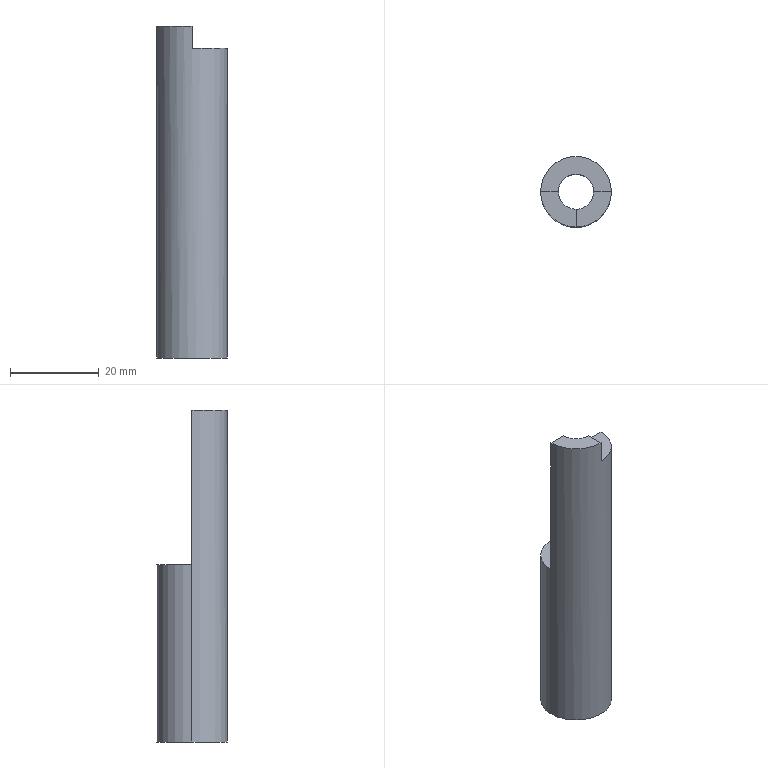Part | CATIA | 1 solid | 11 faces | box 16 x 16 x 75 mm | volume 8482 mm3 | plane 7 | cylinder 4 | commonest cylinder face diameters 8 x2 16 x2
STEP:
#1=CARTESIAN_POINT('',(-8.,0.,13.));
#2=VERTEX_POINT('',#1);
#3=CARTESIAN_POINT('',(8.,0.,13.));
#4=VERTEX_POINT('',#3);
#5=CARTESIAN_POINT('',(0.,0.,13.));
#6=DIRECTION('',(0.,0.,1.));
#7=AXIS2_PLACEMENT_3D('',#5,#6,$);
#8=CIRCLE('',#7,8.);
#9=EDGE_CURVE('',#2,#4,#8,.T.);
#10=ORIENTED_EDGE('',*,*,#9,.F.);
#11=CARTESIAN_POINT('',(0.,0.,13.));
#12=DIRECTION('',(0.,0.,1.));
#13=AXIS2_PLACEMENT_3D('',#11,#12,$);
#14=CIRCLE('',#13,8.);
#15=EDGE_CURVE('',#4,#2,#14,.T.);
#16=ORIENTED_EDGE('',*,*,#15,.F.);
#17=EDGE_LOOP('',(#10,#16));
#18=FACE_OUTER_BOUND('',#17,.T.);
#19=CARTESIAN_POINT('',(4.,0.,13.));
#20=VERTEX_POINT('',#19);
#21=CARTESIAN_POINT('',(-4.,0.,13.));
#22=VERTEX_POINT('',#21);
#23=CARTESIAN_POINT('',(0.,0.,13.));
#24=DIRECTION('',(0.,0.,1.));
#25=AXIS2_PLACEMENT_3D('',#23,#24,$);
#26=CIRCLE('',#25,4.);
#27=EDGE_CURVE('',#20,#22,#26,.T.);
#28=ORIENTED_EDGE('',*,*,#27,.T.);
#29=CARTESIAN_POINT('',(0.,0.,13.));
#30=DIRECTION('',(0.,0.,1.));
#31=AXIS2_PLACEMENT_3D('',#29,#30,$);
#32=CIRCLE('',#31,4.);
#33=EDGE_CURVE('',#22,#20,#32,.T.);
#34=ORIENTED_EDGE('',*,*,#33,.T.);
#35=EDGE_LOOP('',(#28,#34));
#36=FACE_BOUND('',#35,.T.);
#37=CARTESIAN_POINT('',(0.,0.,13.));
#38=DIRECTION('',(0.,0.,1.));
#39=DIRECTION('',(1.,0.,0.));
#40=AXIS2_PLACEMENT_3D('',#37,#38,#39);
#41=PLANE('',#40);
#42=ADVANCED_FACE('',(#18,#36),#41,.F.);
#43=CARTESIAN_POINT('',(4.,0.,53.));
#44=VERTEX_POINT('',#43);
#45=CARTESIAN_POINT('',(-4.,0.,53.));
#46=VERTEX_POINT('',#45);
#47=CARTESIAN_POINT('',(0.,0.,53.));
#48=DIRECTION('',(0.,0.,1.));
#49=AXIS2_PLACEMENT_3D('',#47,#48,$);
#50=CIRCLE('',#49,4.);
#51=EDGE_CURVE('',#44,#46,#50,.T.);
#52=ORIENTED_EDGE('',*,*,#51,.T.);
#53=CARTESIAN_POINT('',(-4.,0.,50.5));
#54=DIRECTION('',(0.,0.,1.));
#55=VECTOR('',#54,1.);
#56=LINE('',#53,#55);
#57=EDGE_CURVE('',#46,#22,#56,.F.);
#58=ORIENTED_EDGE('',*,*,#57,.T.);
#59=ORIENTED_EDGE('',*,*,#27,.F.);
#60=CARTESIAN_POINT('',(4.,0.,50.5));
#61=DIRECTION('',(0.,0.,1.));
#62=VECTOR('',#61,1.);
#63=LINE('',#60,#62);
#64=EDGE_CURVE('',#44,#20,#63,.F.);
#65=ORIENTED_EDGE('',*,*,#64,.F.);
#66=EDGE_LOOP('',(#52,#58,#59,#65));
#67=FACE_OUTER_BOUND('',#66,.T.);
#68=CARTESIAN_POINT('',(0.,0.,50.5));
#69=DIRECTION('',(0.,0.,1.));
#70=DIRECTION('',(1.,0.,0.));
#71=AXIS2_PLACEMENT_3D('',#68,#69,#70);
#72=CYLINDRICAL_SURFACE('',#71,4.);
#73=ADVANCED_FACE('',(#67),#72,.F.);
#74=CARTESIAN_POINT('',(8.,0.,53.));
#75=VERTEX_POINT('',#74);
#76=CARTESIAN_POINT('',(8.,0.,50.5));
#77=DIRECTION('',(0.,0.,1.));
#78=VECTOR('',#77,1.);
#79=LINE('',#76,#78);
#80=EDGE_CURVE('',#75,#4,#79,.F.);
#81=ORIENTED_EDGE('',*,*,#80,.T.);
#82=ORIENTED_EDGE('',*,*,#15,.T.);
#83=CARTESIAN_POINT('',(-8.,0.,53.));
#84=VERTEX_POINT('',#83);
#85=CARTESIAN_POINT('',(-8.,0.,50.5));
#86=DIRECTION('',(0.,0.,1.));
#87=VECTOR('',#86,1.);
#88=LINE('',#85,#87);
#89=EDGE_CURVE('',#84,#2,#88,.F.);
#90=ORIENTED_EDGE('',*,*,#89,.F.);
#91=CARTESIAN_POINT('',(0.,0.,53.));
#92=DIRECTION('',(0.,0.,1.));
#93=AXIS2_PLACEMENT_3D('',#91,#92,$);
#94=CIRCLE('',#93,8.);
#95=EDGE_CURVE('',#75,#84,#94,.T.);
#96=ORIENTED_EDGE('',*,*,#95,.F.);
#97=EDGE_LOOP('',(#81,#82,#90,#96));
#98=FACE_OUTER_BOUND('',#97,.T.);
#99=CARTESIAN_POINT('',(0.,0.,50.5));
#100=DIRECTION('',(0.,0.,1.));
#101=DIRECTION('',(1.,0.,0.));
#102=AXIS2_PLACEMENT_3D('',#99,#100,#101);
#103=CYLINDRICAL_SURFACE('',#102,8.);
#104=ADVANCED_FACE('',(#98),#103,.T.);
#105=ORIENTED_EDGE('',*,*,#51,.F.);
#106=CARTESIAN_POINT('',(6.,0.,53.));
#107=DIRECTION('',(1.,0.,0.));
#108=VECTOR('',#107,1.);
#109=LINE('',#106,#108);
#110=EDGE_CURVE('',#44,#75,#109,.T.);
#111=ORIENTED_EDGE('',*,*,#110,.T.);
#112=ORIENTED_EDGE('',*,*,#95,.T.);
#113=CARTESIAN_POINT('',(-6.,0.,53.));
#114=DIRECTION('',(1.,0.,0.));
#115=VECTOR('',#114,1.);
#116=LINE('',#113,#115);
#117=EDGE_CURVE('',#84,#46,#116,.T.);
#118=ORIENTED_EDGE('',*,*,#117,.T.);
#119=EDGE_LOOP('',(#105,#111,#112,#118));
#120=FACE_OUTER_BOUND('',#119,.T.);
#121=CARTESIAN_POINT('',(0.,0.,53.));
#122=DIRECTION('',(0.,0.,1.));
#123=DIRECTION('',(1.,0.,0.));
#124=AXIS2_PLACEMENT_3D('',#121,#122,#123);
#125=PLANE('',#124);
#126=ADVANCED_FACE('',(#120),#125,.T.);
#127=CARTESIAN_POINT('',(-4.,0.,88.));
#128=VERTEX_POINT('',#127);
#129=CARTESIAN_POINT('',(-4.,0.,70.5));
#130=DIRECTION('',(0.,0.,1.));
#131=VECTOR('',#130,1.);
#132=LINE('',#129,#131);
#133=EDGE_CURVE('',#128,#46,#132,.F.);
#134=ORIENTED_EDGE('',*,*,#133,.T.);
#135=ORIENTED_EDGE('',*,*,#117,.F.);
#136=CARTESIAN_POINT('',(-8.,0.,88.));
#137=VERTEX_POINT('',#136);
#138=CARTESIAN_POINT('',(-8.,0.,70.5));
#139=DIRECTION('',(0.,0.,1.));
#140=VECTOR('',#139,1.);
#141=LINE('',#138,#140);
#142=EDGE_CURVE('',#137,#84,#141,.F.);
#143=ORIENTED_EDGE('',*,*,#142,.F.);
#144=CARTESIAN_POINT('',(-6.,0.,88.));
#145=DIRECTION('',(1.,0.,0.));
#146=VECTOR('',#145,1.);
#147=LINE('',#144,#146);
#148=EDGE_CURVE('',#137,#128,#147,.T.);
#149=ORIENTED_EDGE('',*,*,#148,.T.);
#150=EDGE_LOOP('',(#134,#135,#143,#149));
#151=FACE_OUTER_BOUND('',#150,.T.);
#152=CARTESIAN_POINT('',(-12.734,0.,88.));
#153=DIRECTION('',(0.,1.,0.));
#154=DIRECTION('',(1.,0.,0.));
#155=AXIS2_PLACEMENT_3D('',#152,#153,#154);
#156=PLANE('',#155);
#157=ADVANCED_FACE('',(#151),#156,.T.);
#158=CARTESIAN_POINT('',(8.,0.,83.));
#159=VERTEX_POINT('',#158);
#160=CARTESIAN_POINT('',(8.,0.,68.));
#161=DIRECTION('',(0.,0.,1.));
#162=VECTOR('',#161,1.);
#163=LINE('',#160,#162);
#164=EDGE_CURVE('',#159,#75,#163,.F.);
#165=ORIENTED_EDGE('',*,*,#164,.T.);
#166=ORIENTED_EDGE('',*,*,#110,.F.);
#167=CARTESIAN_POINT('',(4.,0.,83.));
#168=VERTEX_POINT('',#167);
#169=CARTESIAN_POINT('',(4.,0.,68.));
#170=DIRECTION('',(0.,0.,1.));
#171=VECTOR('',#170,1.);
#172=LINE('',#169,#171);
#173=EDGE_CURVE('',#168,#44,#172,.F.);
#174=ORIENTED_EDGE('',*,*,#173,.F.);
#175=CARTESIAN_POINT('',(6.,0.,83.));
#176=DIRECTION('',(1.,0.,0.));
#177=VECTOR('',#176,1.);
#178=LINE('',#175,#177);
#179=EDGE_CURVE('',#168,#159,#178,.T.);
#180=ORIENTED_EDGE('',*,*,#179,.T.);
#181=EDGE_LOOP('',(#165,#166,#174,#180));
#182=FACE_OUTER_BOUND('',#181,.T.);
#183=ADVANCED_FACE('',(#182),#156,.T.);
#184=CARTESIAN_POINT('',(0.,-4.,88.));
#185=VERTEX_POINT('',#184);
#186=CARTESIAN_POINT('',(0.,0.,88.));
#187=DIRECTION('',(0.,0.,1.));
#188=AXIS2_PLACEMENT_3D('',#186,#187,$);
#189=CIRCLE('',#188,4.);
#190=EDGE_CURVE('',#128,#185,#189,.T.);
#191=ORIENTED_EDGE('',*,*,#190,.F.);
#192=ORIENTED_EDGE('',*,*,#148,.F.);
#193=CARTESIAN_POINT('',(0.,-8.,88.));
#194=VERTEX_POINT('',#193);
#195=CARTESIAN_POINT('',(0.,0.,88.));
#196=DIRECTION('',(0.,0.,1.));
#197=AXIS2_PLACEMENT_3D('',#195,#196,$);
#198=CIRCLE('',#197,8.);
#199=EDGE_CURVE('',#137,#194,#198,.T.);
#200=ORIENTED_EDGE('',*,*,#199,.T.);
#201=CARTESIAN_POINT('',(0.,-6.,88.));
#202=DIRECTION('',(0.,-1.,0.));
#203=VECTOR('',#202,1.);
#204=LINE('',#201,#203);
#205=EDGE_CURVE('',#185,#194,#204,.T.);
#206=ORIENTED_EDGE('',*,*,#205,.F.);
#207=EDGE_LOOP('',(#191,#192,#200,#206));
#208=FACE_OUTER_BOUND('',#207,.T.);
#209=CARTESIAN_POINT('',(0.,0.,88.));
#210=DIRECTION('',(0.,0.,1.));
#211=DIRECTION('',(1.,0.,0.));
#212=AXIS2_PLACEMENT_3D('',#209,#210,#211);
#213=PLANE('',#212);
#214=ADVANCED_FACE('',(#208),#213,.T.);
#215=CARTESIAN_POINT('',(0.,-4.,83.));
#216=VERTEX_POINT('',#215);
#217=CARTESIAN_POINT('',(0.,-4.,50.5));
#218=DIRECTION('',(0.,0.,1.));
#219=VECTOR('',#218,1.);
#220=LINE('',#217,#219);
#221=EDGE_CURVE('',#185,#216,#220,.F.);
#222=ORIENTED_EDGE('',*,*,#221,.T.);
#223=CARTESIAN_POINT('',(0.,0.,83.));
#224=DIRECTION('',(0.,0.,1.));
#225=AXIS2_PLACEMENT_3D('',#223,#224,$);
#226=CIRCLE('',#225,4.);
#227=EDGE_CURVE('',#216,#168,#226,.T.);
#228=ORIENTED_EDGE('',*,*,#227,.T.);
#229=ORIENTED_EDGE('',*,*,#173,.T.);
#230=ORIENTED_EDGE('',*,*,#64,.T.);
#231=ORIENTED_EDGE('',*,*,#33,.F.);
#232=ORIENTED_EDGE('',*,*,#57,.F.);
#233=ORIENTED_EDGE('',*,*,#133,.F.);
#234=ORIENTED_EDGE('',*,*,#190,.T.);
#235=EDGE_LOOP('',(#222,#228,#229,#230,#231,#232,#233,#234));
#236=FACE_OUTER_BOUND('',#235,.T.);
#237=ADVANCED_FACE('',(#236),#72,.F.);
#238=ORIENTED_EDGE('',*,*,#199,.F.);
#239=ORIENTED_EDGE('',*,*,#142,.T.);
#240=ORIENTED_EDGE('',*,*,#89,.T.);
#241=ORIENTED_EDGE('',*,*,#9,.T.);
#242=ORIENTED_EDGE('',*,*,#80,.F.);
#243=ORIENTED_EDGE('',*,*,#164,.F.);
#244=CARTESIAN_POINT('',(0.,-8.,83.));
#245=VERTEX_POINT('',#244);
#246=CARTESIAN_POINT('',(0.,0.,83.));
#247=DIRECTION('',(0.,0.,1.));
#248=AXIS2_PLACEMENT_3D('',#246,#247,$);
#249=CIRCLE('',#248,8.);
#250=EDGE_CURVE('',#245,#159,#249,.T.);
#251=ORIENTED_EDGE('',*,*,#250,.F.);
#252=CARTESIAN_POINT('',(0.,-8.,50.5));
#253=DIRECTION('',(0.,0.,1.));
#254=VECTOR('',#253,1.);
#255=LINE('',#252,#254);
#256=EDGE_CURVE('',#194,#245,#255,.F.);
#257=ORIENTED_EDGE('',*,*,#256,.F.);
#258=EDGE_LOOP('',(#238,#239,#240,#241,#242,#243,#251,#257));
#259=FACE_OUTER_BOUND('',#258,.T.);
#260=ADVANCED_FACE('',(#259),#103,.T.);
#261=CARTESIAN_POINT('',(0.,-6.,83.));
#262=DIRECTION('',(0.,-1.,0.));
#263=VECTOR('',#262,1.);
#264=LINE('',#261,#263);
#265=EDGE_CURVE('',#216,#245,#264,.T.);
#266=ORIENTED_EDGE('',*,*,#265,.T.);
#267=ORIENTED_EDGE('',*,*,#250,.T.);
#268=ORIENTED_EDGE('',*,*,#179,.F.);
#269=ORIENTED_EDGE('',*,*,#227,.F.);
#270=EDGE_LOOP('',(#266,#267,#268,#269));
#271=FACE_OUTER_BOUND('',#270,.T.);
#272=CARTESIAN_POINT('',(0.,0.,83.));
#273=DIRECTION('',(0.,0.,1.));
#274=DIRECTION('',(1.,0.,0.));
#275=AXIS2_PLACEMENT_3D('',#272,#273,#274);
#276=PLANE('',#275);
#277=ADVANCED_FACE('',(#271),#276,.T.);
#278=ORIENTED_EDGE('',*,*,#256,.T.);
#279=ORIENTED_EDGE('',*,*,#265,.F.);
#280=ORIENTED_EDGE('',*,*,#221,.F.);
#281=ORIENTED_EDGE('',*,*,#205,.T.);
#282=EDGE_LOOP('',(#278,#279,#280,#281));
#283=FACE_OUTER_BOUND('',#282,.T.);
#284=CARTESIAN_POINT('',(0.,10.,88.));
#285=DIRECTION('',(1.,0.,0.));
#286=DIRECTION('',(0.,-1.,0.));
#287=AXIS2_PLACEMENT_3D('',#284,#285,#286);
#288=PLANE('',#287);
#289=ADVANCED_FACE('',(#283),#288,.T.);
#290=CLOSED_SHELL('',(#42,#73,#104,#126,#157,#183,#214,#237,#260,#277,#289));
#291=MANIFOLD_SOLID_BREP('',#290);
#292=(LENGTH_UNIT()NAMED_UNIT(*)SI_UNIT(.MILLI.,.METRE.));
#293=UNCERTAINTY_MEASURE_WITH_UNIT(LENGTH_MEASURE(0.005),#292,'','');
#294=(NAMED_UNIT(*)PLANE_ANGLE_UNIT()SI_UNIT($,.RADIAN.));
#295=(NAMED_UNIT(*)SI_UNIT($,.STERADIAN.)SOLID_ANGLE_UNIT());
#296=(GEOMETRIC_REPRESENTATION_CONTEXT(3)GLOBAL_UNCERTAINTY_ASSIGNED_CONTEXT((#293))GLOBAL_UNIT_ASSIGNED_CONTEXT((#292,#294,#295))REPRESENTATION_CONTEXT('',''));
#297=ADVANCED_BREP_SHAPE_REPRESENTATION('',(#291),#296);